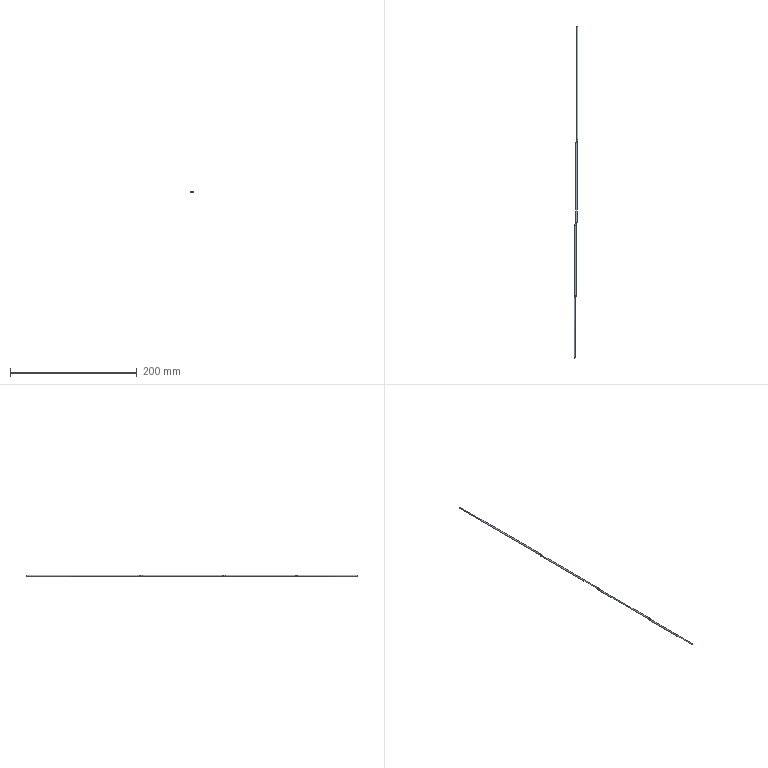Part | STEP file | 1-56.24 | 1 solid | 12 faces | box 5.973 x 524.553 x 2 mm | volume 1650 mm3 | torus 6 | cylinder 4 | plane 2 | commonest cylinder face diameters 2 x4
STEP:
#1=CARTESIAN_POINT('',(0.,0.,0.));
#2=DIRECTION('',(0.,0.,1.));
#3=DIRECTION('',(1.,0.,0.));
#4=AXIS2_PLACEMENT_3D('',#1,#2,#3);
#5=CARTESIAN_POINT('',(1.,0.,0.));
#6=VERTEX_POINT('',#5);
#7=CARTESIAN_POINT('',(0.,0.,0.));
#8=DIRECTION('',(0.,-1.,0.));
#9=DIRECTION('',(1.,0.,0.));
#10=AXIS2_PLACEMENT_3D('',#7,#8,#9);
#11=CIRCLE('',#10,1.);
#12=CARTESIAN_POINT('',(0.,0.,0.));
#13=DIRECTION('',(0.,-1.,0.));
#14=DIRECTION('',(0.,0.,-1.));
#15=AXIS2_PLACEMENT_3D('',#12,#13,#14);
#16=PLANE('',#15);
#17=CARTESIAN_POINT('',(0.,0.));
#18=DIRECTION('',(0.,1.));
#19=AXIS2_PLACEMENT_2D('',#17,#18);
#20=CIRCLE('',#19,1.);
#21=(GEOMETRIC_REPRESENTATION_CONTEXT(2)PARAMETRIC_REPRESENTATION_CONTEXT()REPRESENTATION_CONTEXT('',''));
#22=DEFINITIONAL_REPRESENTATION('',(#20),#21);
#23=PCURVE('',#16,#22);
#24=CARTESIAN_POINT('',(0.,0.,0.));
#25=DIRECTION('',(0.,1.,0.));
#26=DIRECTION('',(1.,0.,0.));
#27=AXIS2_PLACEMENT_3D('',#24,#25,#26);
#28=CYLINDRICAL_SURFACE('',#27,1.);
#29=CARTESIAN_POINT('',(6.283,0.));
#30=DIRECTION('',(-1.,0.));
#31=VECTOR('',#30,1.);
#32=LINE('',#29,#31);
#33=(GEOMETRIC_REPRESENTATION_CONTEXT(2)PARAMETRIC_REPRESENTATION_CONTEXT()REPRESENTATION_CONTEXT('',''));
#34=DEFINITIONAL_REPRESENTATION('',(#32),#33);
#35=PCURVE('',#28,#34);
#36=SURFACE_CURVE('',#11,(#23,#35),.PCURVE_S1.);
#37=EDGE_CURVE('',#6,#6,#36,.T.);
#38=ORIENTED_EDGE('',*,*,#37,.T.);
#39=EDGE_LOOP('',(#38));
#40=FACE_BOUND('',#39,.T.);
#41=ADVANCED_FACE('',(#40),#16,.T.);
#42=CARTESIAN_POINT('',(4.973,524.553,0.));
#43=VERTEX_POINT('',#42);
#44=CARTESIAN_POINT('',(3.973,524.553,0.));
#45=DIRECTION('',(0.,1.,0.));
#46=DIRECTION('',(1.,0.,0.));
#47=AXIS2_PLACEMENT_3D('',#44,#45,#46);
#48=CIRCLE('',#47,1.);
#49=CARTESIAN_POINT('',(3.973,524.553,0.));
#50=DIRECTION('',(0.,1.,0.));
#51=DIRECTION('',(1.,0.,0.));
#52=AXIS2_PLACEMENT_3D('',#49,#50,#51);
#53=PLANE('',#52);
#54=CARTESIAN_POINT('',(0.,0.));
#55=DIRECTION('',(1.,0.));
#56=AXIS2_PLACEMENT_2D('',#54,#55);
#57=CIRCLE('',#56,1.);
#58=(GEOMETRIC_REPRESENTATION_CONTEXT(2)PARAMETRIC_REPRESENTATION_CONTEXT()REPRESENTATION_CONTEXT('',''));
#59=DEFINITIONAL_REPRESENTATION('',(#57),#58);
#60=PCURVE('',#53,#59);
#61=CARTESIAN_POINT('',(3.973,344.553,0.));
#62=DIRECTION('',(0.,1.,0.));
#63=DIRECTION('',(1.,0.,0.));
#64=AXIS2_PLACEMENT_3D('',#61,#62,#63);
#65=CYLINDRICAL_SURFACE('',#64,1.);
#66=CARTESIAN_POINT('',(0.,180.));
#67=DIRECTION('',(1.,0.));
#68=VECTOR('',#67,1.);
#69=LINE('',#66,#68);
#70=(GEOMETRIC_REPRESENTATION_CONTEXT(2)PARAMETRIC_REPRESENTATION_CONTEXT()REPRESENTATION_CONTEXT('',''));
#71=DEFINITIONAL_REPRESENTATION('',(#69),#70);
#72=PCURVE('',#65,#71);
#73=SURFACE_CURVE('',#48,(#60,#72),.PCURVE_S1.);
#74=EDGE_CURVE('',#43,#43,#73,.T.);
#75=ORIENTED_EDGE('',*,*,#74,.T.);
#76=EDGE_LOOP('',(#75));
#77=FACE_BOUND('',#76,.T.);
#78=ADVANCED_FACE('',(#77),#53,.T.);
#79=ORIENTED_EDGE('',*,*,#37,.F.);
#80=CARTESIAN_POINT('',(1.,95.,0.));
#81=VERTEX_POINT('',#80);
#82=CARTESIAN_POINT('',(1.,0.,0.));
#83=DIRECTION('',(0.,1.,0.));
#84=VECTOR('',#83,1.);
#85=LINE('',#82,#84);
#86=CARTESIAN_POINT('',(6.283,0.));
#87=DIRECTION('',(0.,1.));
#88=VECTOR('',#87,1.);
#89=LINE('',#86,#88);
#90=(GEOMETRIC_REPRESENTATION_CONTEXT(2)PARAMETRIC_REPRESENTATION_CONTEXT()REPRESENTATION_CONTEXT('',''));
#91=DEFINITIONAL_REPRESENTATION('',(#89),#90);
#92=PCURVE('',#28,#91);
#93=CARTESIAN_POINT('',(0.,0.));
#94=DIRECTION('',(0.,1.));
#95=VECTOR('',#94,1.);
#96=LINE('',#93,#95);
#97=(GEOMETRIC_REPRESENTATION_CONTEXT(2)PARAMETRIC_REPRESENTATION_CONTEXT()REPRESENTATION_CONTEXT('',''));
#98=DEFINITIONAL_REPRESENTATION('',(#96),#97);
#99=PCURVE('',#28,#98);
#100=SEAM_CURVE('',#85,(#92,#99),.PCURVE_S1.);
#101=EDGE_CURVE('',#6,#81,#100,.T.);
#102=ORIENTED_EDGE('',*,*,#101,.T.);
#103=CARTESIAN_POINT('',(0.,95.,-1.));
#104=VERTEX_POINT('',#103);
#105=CARTESIAN_POINT('',(0.,95.,0.));
#106=DIRECTION('',(0.,1.,0.));
#107=DIRECTION('',(0.,0.,-1.));
#108=AXIS2_PLACEMENT_3D('',#105,#106,#107);
#109=CIRCLE('',#108,1.);
#110=CARTESIAN_POINT('',(1.571,95.));
#111=DIRECTION('',(1.,0.));
#112=VECTOR('',#111,1.);
#113=LINE('',#110,#112);
#114=(GEOMETRIC_REPRESENTATION_CONTEXT(2)PARAMETRIC_REPRESENTATION_CONTEXT()REPRESENTATION_CONTEXT('',''));
#115=DEFINITIONAL_REPRESENTATION('',(#113),#114);
#116=PCURVE('',#28,#115);
#117=CARTESIAN_POINT('',(2.72,95.,0.));
#118=DIRECTION('',(0.,0.,1.));
#119=DIRECTION('',(-1.,0.,0.));
#120=AXIS2_PLACEMENT_3D('',#117,#118,#119);
#121=TOROIDAL_SURFACE('',#120,2.72,1.);
#122=CARTESIAN_POINT('',(6.283,-1.571));
#123=DIRECTION('',(0.,1.));
#124=VECTOR('',#123,1.);
#125=LINE('',#122,#124);
#126=(GEOMETRIC_REPRESENTATION_CONTEXT(2)PARAMETRIC_REPRESENTATION_CONTEXT()REPRESENTATION_CONTEXT('',''));
#127=DEFINITIONAL_REPRESENTATION('',(#125),#126);
#128=PCURVE('',#121,#127);
#129=SURFACE_CURVE('',#109,(#116,#128),.PCURVE_S1.);
#130=EDGE_CURVE('',#104,#81,#129,.T.);
#131=ORIENTED_EDGE('',*,*,#130,.F.);
#132=CARTESIAN_POINT('',(0.,95.,0.));
#133=DIRECTION('',(0.,1.,0.));
#134=DIRECTION('',(1.,0.,0.));
#135=AXIS2_PLACEMENT_3D('',#132,#133,#134);
#136=CIRCLE('',#135,1.);
#137=CARTESIAN_POINT('',(0.,95.));
#138=DIRECTION('',(1.,0.));
#139=VECTOR('',#138,1.);
#140=LINE('',#137,#139);
#141=(GEOMETRIC_REPRESENTATION_CONTEXT(2)PARAMETRIC_REPRESENTATION_CONTEXT()REPRESENTATION_CONTEXT('',''));
#142=DEFINITIONAL_REPRESENTATION('',(#140),#141);
#143=PCURVE('',#28,#142);
#144=CARTESIAN_POINT('',(6.283,3.142));
#145=DIRECTION('',(0.,1.));
#146=VECTOR('',#145,1.);
#147=LINE('',#144,#146);
#148=(GEOMETRIC_REPRESENTATION_CONTEXT(2)PARAMETRIC_REPRESENTATION_CONTEXT()REPRESENTATION_CONTEXT('',''));
#149=DEFINITIONAL_REPRESENTATION('',(#147),#148);
#150=PCURVE('',#121,#149);
#151=SURFACE_CURVE('',#136,(#143,#150),.PCURVE_S1.);
#152=EDGE_CURVE('',#81,#104,#151,.T.);
#153=ORIENTED_EDGE('',*,*,#152,.F.);
#154=ORIENTED_EDGE('',*,*,#101,.F.);
#155=EDGE_LOOP('',(#79,#102,#131,#153,#154));
#156=FACE_BOUND('',#155,.T.);
#157=ADVANCED_FACE('',(#156),#28,.T.);
#158=ORIENTED_EDGE('',*,*,#130,.T.);
#159=ORIENTED_EDGE('',*,*,#152,.T.);
#160=CARTESIAN_POINT('',(0.6313,96.742,-1.));
#161=VERTEX_POINT('',#160);
#162=CARTESIAN_POINT('',(2.72,95.,-1.));
#163=DIRECTION('',(0.,0.,-1.));
#164=DIRECTION('',(-1.,0.,0.));
#165=AXIS2_PLACEMENT_3D('',#162,#163,#164);
#166=CIRCLE('',#165,2.72);
#167=CARTESIAN_POINT('',(6.283,4.712));
#168=DIRECTION('',(-1.,0.));
#169=VECTOR('',#168,1.);
#170=LINE('',#167,#169);
#171=(GEOMETRIC_REPRESENTATION_CONTEXT(2)PARAMETRIC_REPRESENTATION_CONTEXT()REPRESENTATION_CONTEXT('',''));
#172=DEFINITIONAL_REPRESENTATION('',(#170),#171);
#173=PCURVE('',#121,#172);
#174=CARTESIAN_POINT('',(6.283,-1.571));
#175=DIRECTION('',(-1.,0.));
#176=VECTOR('',#175,1.);
#177=LINE('',#174,#176);
#178=(GEOMETRIC_REPRESENTATION_CONTEXT(2)PARAMETRIC_REPRESENTATION_CONTEXT()REPRESENTATION_CONTEXT('',''));
#179=DEFINITIONAL_REPRESENTATION('',(#177),#178);
#180=PCURVE('',#121,#179);
#181=SEAM_CURVE('',#166,(#173,#180),.PCURVE_S1.);
#182=EDGE_CURVE('',#104,#161,#181,.T.);
#183=ORIENTED_EDGE('',*,*,#182,.T.);
#184=CARTESIAN_POINT('',(0.6313,96.742,0.));
#185=DIRECTION('',(-0.6406,-0.7679,0.));
#186=DIRECTION('',(0.,0.,-1.));
#187=AXIS2_PLACEMENT_3D('',#184,#185,#186);
#188=CIRCLE('',#187,1.);
#189=CARTESIAN_POINT('',(5.588,4.712));
#190=DIRECTION('',(0.,-1.));
#191=VECTOR('',#190,1.);
#192=LINE('',#189,#191);
#193=(GEOMETRIC_REPRESENTATION_CONTEXT(2)PARAMETRIC_REPRESENTATION_CONTEXT()REPRESENTATION_CONTEXT('',''));
#194=DEFINITIONAL_REPRESENTATION('',(#192),#193);
#195=PCURVE('',#121,#194);
#196=CARTESIAN_POINT('',(-1.301,98.354,0.));
#197=DIRECTION('',(0.,0.,-1.));
#198=DIRECTION('',(0.7679,-0.6406,0.));
#199=AXIS2_PLACEMENT_3D('',#196,#197,#198);
#200=TOROIDAL_SURFACE('',#199,2.516,1.);
#201=CARTESIAN_POINT('',(6.283,7.854));
#202=DIRECTION('',(0.,-1.));
#203=VECTOR('',#202,1.);
#204=LINE('',#201,#203);
#205=(GEOMETRIC_REPRESENTATION_CONTEXT(2)PARAMETRIC_REPRESENTATION_CONTEXT()REPRESENTATION_CONTEXT('',''));
#206=DEFINITIONAL_REPRESENTATION('',(#204),#205);
#207=PCURVE('',#200,#206);
#208=SURFACE_CURVE('',#188,(#195,#207),.PCURVE_S1.);
#209=EDGE_CURVE('',#161,#161,#208,.T.);
#210=ORIENTED_EDGE('',*,*,#209,.T.);
#211=ORIENTED_EDGE('',*,*,#182,.F.);
#212=EDGE_LOOP('',(#158,#159,#183,#210,#211));
#213=FACE_BOUND('',#212,.T.);
#214=ADVANCED_FACE('',(#213),#121,.T.);
#215=ORIENTED_EDGE('',*,*,#209,.F.);
#216=CARTESIAN_POINT('',(1.215,98.354,-1.));
#217=VERTEX_POINT('',#216);
#218=CARTESIAN_POINT('',(-1.301,98.354,-1.));
#219=DIRECTION('',(0.,0.,1.));
#220=DIRECTION('',(0.7679,-0.6406,0.));
#221=AXIS2_PLACEMENT_3D('',#218,#219,#220);
#222=CIRCLE('',#221,2.516);
#223=CARTESIAN_POINT('',(6.283,7.854));
#224=DIRECTION('',(-1.,0.));
#225=VECTOR('',#224,1.);
#226=LINE('',#223,#225);
#227=(GEOMETRIC_REPRESENTATION_CONTEXT(2)PARAMETRIC_REPRESENTATION_CONTEXT()REPRESENTATION_CONTEXT('',''));
#228=DEFINITIONAL_REPRESENTATION('',(#226),#227);
#229=PCURVE('',#200,#228);
#230=CARTESIAN_POINT('',(6.283,1.571));
#231=DIRECTION('',(-1.,0.));
#232=VECTOR('',#231,1.);
#233=LINE('',#230,#232);
#234=(GEOMETRIC_REPRESENTATION_CONTEXT(2)PARAMETRIC_REPRESENTATION_CONTEXT()REPRESENTATION_CONTEXT('',''));
#235=DEFINITIONAL_REPRESENTATION('',(#233),#234);
#236=PCURVE('',#200,#235);
#237=SEAM_CURVE('',#222,(#229,#236),.PCURVE_S1.);
#238=EDGE_CURVE('',#161,#217,#237,.T.);
#239=ORIENTED_EDGE('',*,*,#238,.T.);
#240=CARTESIAN_POINT('',(2.215,98.354,0.));
#241=VERTEX_POINT('',#240);
#242=CARTESIAN_POINT('',(1.215,98.354,0.));
#243=DIRECTION('',(0.,-1.,0.));
#244=DIRECTION('',(0.,0.,-1.));
#245=AXIS2_PLACEMENT_3D('',#242,#243,#244);
#246=CIRCLE('',#245,1.);
#247=CARTESIAN_POINT('',(5.588,7.854));
#248=DIRECTION('',(0.,-1.));
#249=VECTOR('',#248,1.);
#250=LINE('',#247,#249);
#251=(GEOMETRIC_REPRESENTATION_CONTEXT(2)PARAMETRIC_REPRESENTATION_CONTEXT()REPRESENTATION_CONTEXT('',''));
#252=DEFINITIONAL_REPRESENTATION('',(#250),#251);
#253=PCURVE('',#200,#252);
#254=CARTESIAN_POINT('',(1.215,98.354,0.));
#255=DIRECTION('',(0.,1.,0.));
#256=DIRECTION('',(1.,0.,0.));
#257=AXIS2_PLACEMENT_3D('',#254,#255,#256);
#258=CYLINDRICAL_SURFACE('',#257,1.);
#259=CARTESIAN_POINT('',(1.571,0.));
#260=DIRECTION('',(-1.,0.));
#261=VECTOR('',#260,1.);
#262=LINE('',#259,#261);
#263=(GEOMETRIC_REPRESENTATION_CONTEXT(2)PARAMETRIC_REPRESENTATION_CONTEXT()REPRESENTATION_CONTEXT('',''));
#264=DEFINITIONAL_REPRESENTATION('',(#262),#263);
#265=PCURVE('',#258,#264);
#266=SURFACE_CURVE('',#246,(#253,#265),.PCURVE_S1.);
#267=EDGE_CURVE('',#217,#241,#266,.T.);
#268=ORIENTED_EDGE('',*,*,#267,.T.);
#269=CARTESIAN_POINT('',(1.215,98.354,0.));
#270=DIRECTION('',(0.,-1.,0.));
#271=DIRECTION('',(1.,0.,0.));
#272=AXIS2_PLACEMENT_3D('',#269,#270,#271);
#273=CIRCLE('',#272,1.);
#274=CARTESIAN_POINT('',(5.588,6.283));
#275=DIRECTION('',(0.,-1.));
#276=VECTOR('',#275,1.);
#277=LINE('',#274,#276);
#278=(GEOMETRIC_REPRESENTATION_CONTEXT(2)PARAMETRIC_REPRESENTATION_CONTEXT()REPRESENTATION_CONTEXT('',''));
#279=DEFINITIONAL_REPRESENTATION('',(#277),#278);
#280=PCURVE('',#200,#279);
#281=CARTESIAN_POINT('',(6.283,0.));
#282=DIRECTION('',(-1.,0.));
#283=VECTOR('',#282,1.);
#284=LINE('',#281,#283);
#285=(GEOMETRIC_REPRESENTATION_CONTEXT(2)PARAMETRIC_REPRESENTATION_CONTEXT()REPRESENTATION_CONTEXT('',''));
#286=DEFINITIONAL_REPRESENTATION('',(#284),#285);
#287=PCURVE('',#258,#286);
#288=SURFACE_CURVE('',#273,(#280,#287),.PCURVE_S1.);
#289=EDGE_CURVE('',#241,#217,#288,.T.);
#290=ORIENTED_EDGE('',*,*,#289,.T.);
#291=ORIENTED_EDGE('',*,*,#238,.F.);
#292=EDGE_LOOP('',(#215,#239,#268,#290,#291));
#293=FACE_BOUND('',#292,.T.);
#294=ADVANCED_FACE('',(#293),#200,.T.);
#295=ORIENTED_EDGE('',*,*,#267,.F.);
#296=ORIENTED_EDGE('',*,*,#289,.F.);
#297=CARTESIAN_POINT('',(2.215,210.,0.));
#298=VERTEX_POINT('',#297);
#299=CARTESIAN_POINT('',(2.215,98.354,0.));
#300=DIRECTION('',(0.,1.,0.));
#301=VECTOR('',#300,1.);
#302=LINE('',#299,#301);
#303=CARTESIAN_POINT('',(6.283,0.));
#304=DIRECTION('',(0.,1.));
#305=VECTOR('',#304,1.);
#306=LINE('',#303,#305);
#307=(GEOMETRIC_REPRESENTATION_CONTEXT(2)PARAMETRIC_REPRESENTATION_CONTEXT()REPRESENTATION_CONTEXT('',''));
#308=DEFINITIONAL_REPRESENTATION('',(#306),#307);
#309=PCURVE('',#258,#308);
#310=CARTESIAN_POINT('',(0.,0.));
#311=DIRECTION('',(0.,1.));
#312=VECTOR('',#311,1.);
#313=LINE('',#310,#312);
#314=(GEOMETRIC_REPRESENTATION_CONTEXT(2)PARAMETRIC_REPRESENTATION_CONTEXT()REPRESENTATION_CONTEXT('',''));
#315=DEFINITIONAL_REPRESENTATION('',(#313),#314);
#316=PCURVE('',#258,#315);
#317=SEAM_CURVE('',#302,(#309,#316),.PCURVE_S1.);
#318=EDGE_CURVE('',#241,#298,#317,.T.);
#319=ORIENTED_EDGE('',*,*,#318,.T.);
#320=CARTESIAN_POINT('',(1.215,210.,-1.));
#321=VERTEX_POINT('',#320);
#322=CARTESIAN_POINT('',(1.215,210.,0.));
#323=DIRECTION('',(0.,1.,0.));
#324=DIRECTION('',(0.,0.,-1.));
#325=AXIS2_PLACEMENT_3D('',#322,#323,#324);
#326=CIRCLE('',#325,1.);
#327=CARTESIAN_POINT('',(1.571,111.646));
#328=DIRECTION('',(1.,0.));
#329=VECTOR('',#328,1.);
#330=LINE('',#327,#329);
#331=(GEOMETRIC_REPRESENTATION_CONTEXT(2)PARAMETRIC_REPRESENTATION_CONTEXT()REPRESENTATION_CONTEXT('',''));
#332=DEFINITIONAL_REPRESENTATION('',(#330),#331);
#333=PCURVE('',#258,#332);
#334=CARTESIAN_POINT('',(5.335,210.,0.));
#335=DIRECTION('',(0.,0.,1.));
#336=DIRECTION('',(-1.,0.,0.));
#337=AXIS2_PLACEMENT_3D('',#334,#335,#336);
#338=TOROIDAL_SURFACE('',#337,4.12,1.);
#339=CARTESIAN_POINT('',(6.283,-1.571));
#340=DIRECTION('',(0.,1.));
#341=VECTOR('',#340,1.);
#342=LINE('',#339,#341);
#343=(GEOMETRIC_REPRESENTATION_CONTEXT(2)PARAMETRIC_REPRESENTATION_CONTEXT()REPRESENTATION_CONTEXT('',''));
#344=DEFINITIONAL_REPRESENTATION('',(#342),#343);
#345=PCURVE('',#338,#344);
#346=SURFACE_CURVE('',#326,(#333,#345),.PCURVE_S1.);
#347=EDGE_CURVE('',#321,#298,#346,.T.);
#348=ORIENTED_EDGE('',*,*,#347,.F.);
#349=CARTESIAN_POINT('',(1.215,210.,0.));
#350=DIRECTION('',(0.,1.,0.));
#351=DIRECTION('',(1.,0.,0.));
#352=AXIS2_PLACEMENT_3D('',#349,#350,#351);
#353=CIRCLE('',#352,1.);
#354=CARTESIAN_POINT('',(0.,111.646));
#355=DIRECTION('',(1.,0.));
#356=VECTOR('',#355,1.);
#357=LINE('',#354,#356);
#358=(GEOMETRIC_REPRESENTATION_CONTEXT(2)PARAMETRIC_REPRESENTATION_CONTEXT()REPRESENTATION_CONTEXT('',''));
#359=DEFINITIONAL_REPRESENTATION('',(#357),#358);
#360=PCURVE('',#258,#359);
#361=CARTESIAN_POINT('',(6.283,3.142));
#362=DIRECTION('',(0.,1.));
#363=VECTOR('',#362,1.);
#364=LINE('',#361,#363);
#365=(GEOMETRIC_REPRESENTATION_CONTEXT(2)PARAMETRIC_REPRESENTATION_CONTEXT()REPRESENTATION_CONTEXT('',''));
#366=DEFINITIONAL_REPRESENTATION('',(#364),#365);
#367=PCURVE('',#338,#366);
#368=SURFACE_CURVE('',#353,(#360,#367),.PCURVE_S1.);
#369=EDGE_CURVE('',#298,#321,#368,.T.);
#370=ORIENTED_EDGE('',*,*,#369,.F.);
#371=ORIENTED_EDGE('',*,*,#318,.F.);
#372=EDGE_LOOP('',(#295,#296,#319,#348,#370,#371));
#373=FACE_BOUND('',#372,.T.);
#374=ADVANCED_FACE('',(#373),#258,.T.);
#375=ORIENTED_EDGE('',*,*,#347,.T.);
#376=ORIENTED_EDGE('',*,*,#369,.T.);
#377=CARTESIAN_POINT('',(1.87,212.228,-1.));
#378=VERTEX_POINT('',#377);
#379=CARTESIAN_POINT('',(5.335,210.,-1.));
#380=DIRECTION('',(0.,0.,-1.));
#381=DIRECTION('',(-1.,0.,0.));
#382=AXIS2_PLACEMENT_3D('',#379,#380,#381);
#383=CIRCLE('',#382,4.12);
#384=CARTESIAN_POINT('',(6.283,4.712));
#385=DIRECTION('',(-1.,0.));
#386=VECTOR('',#385,1.);
#387=LINE('',#384,#386);
#388=(GEOMETRIC_REPRESENTATION_CONTEXT(2)PARAMETRIC_REPRESENTATION_CONTEXT()REPRESENTATION_CONTEXT('',''));
#389=DEFINITIONAL_REPRESENTATION('',(#387),#388);
#390=PCURVE('',#338,#389);
#391=CARTESIAN_POINT('',(6.283,-1.571));
#392=DIRECTION('',(-1.,0.));
#393=VECTOR('',#392,1.);
#394=LINE('',#391,#393);
#395=(GEOMETRIC_REPRESENTATION_CONTEXT(2)PARAMETRIC_REPRESENTATION_CONTEXT()REPRESENTATION_CONTEXT('',''));
#396=DEFINITIONAL_REPRESENTATION('',(#394),#395);
#397=PCURVE('',#338,#396);
#398=SEAM_CURVE('',#383,(#390,#397),.PCURVE_S1.);
#399=EDGE_CURVE('',#321,#378,#398,.T.);
#400=ORIENTED_EDGE('',*,*,#399,.T.);
#401=CARTESIAN_POINT('',(1.87,212.228,0.));
#402=DIRECTION('',(-0.5407,-0.8412,0.));
#403=DIRECTION('',(0.,0.,-1.));
#404=AXIS2_PLACEMENT_3D('',#401,#402,#403);
#405=CIRCLE('',#404,1.);
#406=CARTESIAN_POINT('',(5.712,4.712));
#407=DIRECTION('',(0.,-1.));
#408=VECTOR('',#407,1.);
#409=LINE('',#406,#408);
#410=(GEOMETRIC_REPRESENTATION_CONTEXT(2)PARAMETRIC_REPRESENTATION_CONTEXT()REPRESENTATION_CONTEXT('',''));
#411=DEFINITIONAL_REPRESENTATION('',(#409),#410);
#412=PCURVE('',#338,#411);
#413=CARTESIAN_POINT('',(-2.211,214.851,0.));
#414=DIRECTION('',(0.,0.,-1.));
#415=DIRECTION('',(0.8412,-0.5407,0.));
#416=AXIS2_PLACEMENT_3D('',#413,#414,#415);
#417=TOROIDAL_SURFACE('',#416,4.851,1.);
#418=CARTESIAN_POINT('',(6.283,7.854));
#419=DIRECTION('',(0.,-1.));
#420=VECTOR('',#419,1.);
#421=LINE('',#418,#420);
#422=(GEOMETRIC_REPRESENTATION_CONTEXT(2)PARAMETRIC_REPRESENTATION_CONTEXT()REPRESENTATION_CONTEXT('',''));
#423=DEFINITIONAL_REPRESENTATION('',(#421),#422);
#424=PCURVE('',#417,#423);
#425=SURFACE_CURVE('',#405,(#412,#424),.PCURVE_S1.);
#426=EDGE_CURVE('',#378,#378,#425,.T.);
#427=ORIENTED_EDGE('',*,*,#426,.T.);
#428=ORIENTED_EDGE('',*,*,#399,.F.);
#429=EDGE_LOOP('',(#375,#376,#400,#427,#428));
#430=FACE_BOUND('',#429,.T.);
#431=ADVANCED_FACE('',(#430),#338,.T.);
#432=ORIENTED_EDGE('',*,*,#426,.F.);
#433=CARTESIAN_POINT('',(2.64,214.851,-1.));
#434=VERTEX_POINT('',#433);
#435=CARTESIAN_POINT('',(-2.211,214.851,-1.));
#436=DIRECTION('',(0.,0.,1.));
#437=DIRECTION('',(0.8412,-0.5407,0.));
#438=AXIS2_PLACEMENT_3D('',#435,#436,#437);
#439=CIRCLE('',#438,4.851);
#440=CARTESIAN_POINT('',(6.283,7.854));
#441=DIRECTION('',(-1.,0.));
#442=VECTOR('',#441,1.);
#443=LINE('',#440,#442);
#444=(GEOMETRIC_REPRESENTATION_CONTEXT(2)PARAMETRIC_REPRESENTATION_CONTEXT()REPRESENTATION_CONTEXT('',''));
#445=DEFINITIONAL_REPRESENTATION('',(#443),#444);
#446=PCURVE('',#417,#445);
#447=CARTESIAN_POINT('',(6.283,1.571));
#448=DIRECTION('',(-1.,0.));
#449=VECTOR('',#448,1.);
#450=LINE('',#447,#449);
#451=(GEOMETRIC_REPRESENTATION_CONTEXT(2)PARAMETRIC_REPRESENTATION_CONTEXT()REPRESENTATION_CONTEXT('',''));
#452=DEFINITIONAL_REPRESENTATION('',(#450),#451);
#453=PCURVE('',#417,#452);
#454=SEAM_CURVE('',#439,(#446,#453),.PCURVE_S1.);
#455=EDGE_CURVE('',#378,#434,#454,.T.);
#456=ORIENTED_EDGE('',*,*,#455,.T.);
#457=CARTESIAN_POINT('',(3.64,214.851,0.));
#458=VERTEX_POINT('',#457);
#459=CARTESIAN_POINT('',(2.64,214.851,0.));
#460=DIRECTION('',(0.,-1.,0.));
#461=DIRECTION('',(0.,0.,-1.));
#462=AXIS2_PLACEMENT_3D('',#459,#460,#461);
#463=CIRCLE('',#462,1.);
#464=CARTESIAN_POINT('',(5.712,7.854));
#465=DIRECTION('',(0.,-1.));
#466=VECTOR('',#465,1.);
#467=LINE('',#464,#466);
#468=(GEOMETRIC_REPRESENTATION_CONTEXT(2)PARAMETRIC_REPRESENTATION_CONTEXT()REPRESENTATION_CONTEXT('',''));
#469=DEFINITIONAL_REPRESENTATION('',(#467),#468);
#470=PCURVE('',#417,#469);
#471=CARTESIAN_POINT('',(2.64,214.851,0.));
#472=DIRECTION('',(0.,1.,0.));
#473=DIRECTION('',(1.,0.,0.));
#474=AXIS2_PLACEMENT_3D('',#471,#472,#473);
#475=CYLINDRICAL_SURFACE('',#474,1.);
#476=CARTESIAN_POINT('',(1.571,0.));
#477=DIRECTION('',(-1.,0.));
#478=VECTOR('',#477,1.);
#479=LINE('',#476,#478);
#480=(GEOMETRIC_REPRESENTATION_CONTEXT(2)PARAMETRIC_REPRESENTATION_CONTEXT()REPRESENTATION_CONTEXT('',''));
#481=DEFINITIONAL_REPRESENTATION('',(#479),#480);
#482=PCURVE('',#475,#481);
#483=SURFACE_CURVE('',#463,(#470,#482),.PCURVE_S1.);
#484=EDGE_CURVE('',#434,#458,#483,.T.);
#485=ORIENTED_EDGE('',*,*,#484,.T.);
#486=CARTESIAN_POINT('',(2.64,214.851,0.));
#487=DIRECTION('',(0.,-1.,0.));
#488=DIRECTION('',(1.,0.,0.));
#489=AXIS2_PLACEMENT_3D('',#486,#487,#488);
#490=CIRCLE('',#489,1.);
#491=CARTESIAN_POINT('',(5.712,6.283));
#492=DIRECTION('',(0.,-1.));
#493=VECTOR('',#492,1.);
#494=LINE('',#491,#493);
#495=(GEOMETRIC_REPRESENTATION_CONTEXT(2)PARAMETRIC_REPRESENTATION_CONTEXT()REPRESENTATION_CONTEXT('',''));
#496=DEFINITIONAL_REPRESENTATION('',(#494),#495);
#497=PCURVE('',#417,#496);
#498=CARTESIAN_POINT('',(6.283,0.));
#499=DIRECTION('',(-1.,0.));
#500=VECTOR('',#499,1.);
#501=LINE('',#498,#500);
#502=(GEOMETRIC_REPRESENTATION_CONTEXT(2)PARAMETRIC_REPRESENTATION_CONTEXT()REPRESENTATION_CONTEXT('',''));
#503=DEFINITIONAL_REPRESENTATION('',(#501),#502);
#504=PCURVE('',#475,#503);
#505=SURFACE_CURVE('',#490,(#497,#504),.PCURVE_S1.);
#506=EDGE_CURVE('',#458,#434,#505,.T.);
#507=ORIENTED_EDGE('',*,*,#506,.T.);
#508=ORIENTED_EDGE('',*,*,#455,.F.);
#509=EDGE_LOOP('',(#432,#456,#485,#507,#508));
#510=FACE_BOUND('',#509,.T.);
#511=ADVANCED_FACE('',(#510),#417,.T.);
#512=ORIENTED_EDGE('',*,*,#484,.F.);
#513=ORIENTED_EDGE('',*,*,#506,.F.);
#514=CARTESIAN_POINT('',(3.64,339.851,0.));
#515=VERTEX_POINT('',#514);
#516=CARTESIAN_POINT('',(3.64,214.851,0.));
#517=DIRECTION('',(0.,1.,0.));
#518=VECTOR('',#517,1.);
#519=LINE('',#516,#518);
#520=CARTESIAN_POINT('',(6.283,0.));
#521=DIRECTION('',(0.,1.));
#522=VECTOR('',#521,1.);
#523=LINE('',#520,#522);
#524=(GEOMETRIC_REPRESENTATION_CONTEXT(2)PARAMETRIC_REPRESENTATION_CONTEXT()REPRESENTATION_CONTEXT('',''));
#525=DEFINITIONAL_REPRESENTATION('',(#523),#524);
#526=PCURVE('',#475,#525);
#527=CARTESIAN_POINT('',(0.,0.));
#528=DIRECTION('',(0.,1.));
#529=VECTOR('',#528,1.);
#530=LINE('',#527,#529);
#531=(GEOMETRIC_REPRESENTATION_CONTEXT(2)PARAMETRIC_REPRESENTATION_CONTEXT()REPRESENTATION_CONTEXT('',''));
#532=DEFINITIONAL_REPRESENTATION('',(#530),#531);
#533=PCURVE('',#475,#532);
#534=SEAM_CURVE('',#519,(#526,#533),.PCURVE_S1.);
#535=EDGE_CURVE('',#458,#515,#534,.T.);
#536=ORIENTED_EDGE('',*,*,#535,.T.);
#537=CARTESIAN_POINT('',(2.64,339.851,-1.));
#538=VERTEX_POINT('',#537);
#539=CARTESIAN_POINT('',(2.64,339.851,0.));
#540=DIRECTION('',(0.,1.,0.));
#541=DIRECTION('',(0.,0.,-1.));
#542=AXIS2_PLACEMENT_3D('',#539,#540,#541);
#543=CIRCLE('',#542,1.);
#544=CARTESIAN_POINT('',(1.571,125.));
#545=DIRECTION('',(1.,0.));
#546=VECTOR('',#545,1.);
#547=LINE('',#544,#546);
#548=(GEOMETRIC_REPRESENTATION_CONTEXT(2)PARAMETRIC_REPRESENTATION_CONTEXT()REPRESENTATION_CONTEXT('',''));
#549=DEFINITIONAL_REPRESENTATION('',(#547),#548);
#550=PCURVE('',#475,#549);
#551=CARTESIAN_POINT('',(7.673,339.851,0.));
#552=DIRECTION('',(0.,0.,1.));
#553=DIRECTION('',(-1.,0.,0.));
#554=AXIS2_PLACEMENT_3D('',#551,#552,#553);
#555=TOROIDAL_SURFACE('',#554,5.033,1.);
#556=CARTESIAN_POINT('',(6.283,-1.571));
#557=DIRECTION('',(0.,1.));
#558=VECTOR('',#557,1.);
#559=LINE('',#556,#558);
#560=(GEOMETRIC_REPRESENTATION_CONTEXT(2)PARAMETRIC_REPRESENTATION_CONTEXT()REPRESENTATION_CONTEXT('',''));
#561=DEFINITIONAL_REPRESENTATION('',(#559),#560);
#562=PCURVE('',#555,#561);
#563=SURFACE_CURVE('',#543,(#550,#562),.PCURVE_S1.);
#564=EDGE_CURVE('',#538,#515,#563,.T.);
#565=ORIENTED_EDGE('',*,*,#564,.F.);
#566=CARTESIAN_POINT('',(2.64,339.851,0.));
#567=DIRECTION('',(0.,1.,0.));
#568=DIRECTION('',(1.,0.,0.));
#569=AXIS2_PLACEMENT_3D('',#566,#567,#568);
#570=CIRCLE('',#569,1.);
#571=CARTESIAN_POINT('',(0.,125.));
#572=DIRECTION('',(1.,0.));
#573=VECTOR('',#572,1.);
#574=LINE('',#571,#573);
#575=(GEOMETRIC_REPRESENTATION_CONTEXT(2)PARAMETRIC_REPRESENTATION_CONTEXT()REPRESENTATION_CONTEXT('',''));
#576=DEFINITIONAL_REPRESENTATION('',(#574),#575);
#577=PCURVE('',#475,#576);
#578=CARTESIAN_POINT('',(6.283,3.142));
#579=DIRECTION('',(0.,1.));
#580=VECTOR('',#579,1.);
#581=LINE('',#578,#580);
#582=(GEOMETRIC_REPRESENTATION_CONTEXT(2)PARAMETRIC_REPRESENTATION_CONTEXT()REPRESENTATION_CONTEXT('',''));
#583=DEFINITIONAL_REPRESENTATION('',(#581),#582);
#584=PCURVE('',#555,#583);
#585=SURFACE_CURVE('',#570,(#577,#584),.PCURVE_S1.);
#586=EDGE_CURVE('',#515,#538,#585,.T.);
#587=ORIENTED_EDGE('',*,*,#586,.F.);
#588=ORIENTED_EDGE('',*,*,#535,.F.);
#589=EDGE_LOOP('',(#512,#513,#536,#565,#587,#588));
#590=FACE_BOUND('',#589,.T.);
#591=ADVANCED_FACE('',(#590),#475,.T.);
#592=ORIENTED_EDGE('',*,*,#564,.T.);
#593=ORIENTED_EDGE('',*,*,#586,.T.);
#594=CARTESIAN_POINT('',(3.389,342.492,-1.));
#595=VERTEX_POINT('',#594);
#596=CARTESIAN_POINT('',(7.673,339.851,-1.));
#597=DIRECTION('',(0.,0.,-1.));
#598=DIRECTION('',(-1.,0.,0.));
#599=AXIS2_PLACEMENT_3D('',#596,#597,#598);
#600=CIRCLE('',#599,5.033);
#601=CARTESIAN_POINT('',(6.283,4.712));
#602=DIRECTION('',(-1.,0.));
#603=VECTOR('',#602,1.);
#604=LINE('',#601,#603);
#605=(GEOMETRIC_REPRESENTATION_CONTEXT(2)PARAMETRIC_REPRESENTATION_CONTEXT()REPRESENTATION_CONTEXT('',''));
#606=DEFINITIONAL_REPRESENTATION('',(#604),#605);
#607=PCURVE('',#555,#606);
#608=CARTESIAN_POINT('',(6.283,-1.571));
#609=DIRECTION('',(-1.,0.));
#610=VECTOR('',#609,1.);
#611=LINE('',#608,#610);
#612=(GEOMETRIC_REPRESENTATION_CONTEXT(2)PARAMETRIC_REPRESENTATION_CONTEXT()REPRESENTATION_CONTEXT('',''));
#613=DEFINITIONAL_REPRESENTATION('',(#611),#612);
#614=PCURVE('',#555,#613);
#615=SEAM_CURVE('',#600,(#607,#614),.PCURVE_S1.);
#616=EDGE_CURVE('',#538,#595,#615,.T.);
#617=ORIENTED_EDGE('',*,*,#616,.T.);
#618=CARTESIAN_POINT('',(3.389,342.492,0.));
#619=DIRECTION('',(-0.5247,-0.8513,0.));
#620=DIRECTION('',(0.,0.,-1.));
#621=AXIS2_PLACEMENT_3D('',#618,#619,#620);
#622=CIRCLE('',#621,1.);
#623=CARTESIAN_POINT('',(5.731,4.712));
#624=DIRECTION('',(0.,-1.));
#625=VECTOR('',#624,1.);
#626=LINE('',#623,#625);
#627=(GEOMETRIC_REPRESENTATION_CONTEXT(2)PARAMETRIC_REPRESENTATION_CONTEXT()REPRESENTATION_CONTEXT('',''));
#628=DEFINITIONAL_REPRESENTATION('',(#626),#627);
#629=PCURVE('',#555,#628);
#630=CARTESIAN_POINT('',(0.04353,344.553,0.));
#631=DIRECTION('',(0.,0.,-1.));
#632=DIRECTION('',(0.8513,-0.5247,0.));
#633=AXIS2_PLACEMENT_3D('',#630,#631,#632);
#634=TOROIDAL_SURFACE('',#633,3.929,1.);
#635=CARTESIAN_POINT('',(6.283,7.854));
#636=DIRECTION('',(0.,-1.));
#637=VECTOR('',#636,1.);
#638=LINE('',#635,#637);
#639=(GEOMETRIC_REPRESENTATION_CONTEXT(2)PARAMETRIC_REPRESENTATION_CONTEXT()REPRESENTATION_CONTEXT('',''));
#640=DEFINITIONAL_REPRESENTATION('',(#638),#639);
#641=PCURVE('',#634,#640);
#642=SURFACE_CURVE('',#622,(#629,#641),.PCURVE_S1.);
#643=EDGE_CURVE('',#595,#595,#642,.T.);
#644=ORIENTED_EDGE('',*,*,#643,.T.);
#645=ORIENTED_EDGE('',*,*,#616,.F.);
#646=EDGE_LOOP('',(#592,#593,#617,#644,#645));
#647=FACE_BOUND('',#646,.T.);
#648=ADVANCED_FACE('',(#647),#555,.T.);
#649=ORIENTED_EDGE('',*,*,#643,.F.);
#650=CARTESIAN_POINT('',(3.973,344.553,-1.));
#651=VERTEX_POINT('',#650);
#652=CARTESIAN_POINT('',(0.04353,344.553,-1.));
#653=DIRECTION('',(0.,0.,1.));
#654=DIRECTION('',(0.8513,-0.5247,0.));
#655=AXIS2_PLACEMENT_3D('',#652,#653,#654);
#656=CIRCLE('',#655,3.929);
#657=CARTESIAN_POINT('',(6.283,7.854));
#658=DIRECTION('',(-1.,0.));
#659=VECTOR('',#658,1.);
#660=LINE('',#657,#659);
#661=(GEOMETRIC_REPRESENTATION_CONTEXT(2)PARAMETRIC_REPRESENTATION_CONTEXT()REPRESENTATION_CONTEXT('',''));
#662=DEFINITIONAL_REPRESENTATION('',(#660),#661);
#663=PCURVE('',#634,#662);
#664=CARTESIAN_POINT('',(6.283,1.571));
#665=DIRECTION('',(-1.,0.));
#666=VECTOR('',#665,1.);
#667=LINE('',#664,#666);
#668=(GEOMETRIC_REPRESENTATION_CONTEXT(2)PARAMETRIC_REPRESENTATION_CONTEXT()REPRESENTATION_CONTEXT('',''));
#669=DEFINITIONAL_REPRESENTATION('',(#667),#668);
#670=PCURVE('',#634,#669);
#671=SEAM_CURVE('',#656,(#663,#670),.PCURVE_S1.);
#672=EDGE_CURVE('',#595,#651,#671,.T.);
#673=ORIENTED_EDGE('',*,*,#672,.T.);
#674=CARTESIAN_POINT('',(4.973,344.553,0.));
#675=VERTEX_POINT('',#674);
#676=CARTESIAN_POINT('',(3.973,344.553,0.));
#677=DIRECTION('',(0.,-1.,0.));
#678=DIRECTION('',(0.,0.,-1.));
#679=AXIS2_PLACEMENT_3D('',#676,#677,#678);
#680=CIRCLE('',#679,1.);
#681=CARTESIAN_POINT('',(5.731,7.854));
#682=DIRECTION('',(0.,-1.));
#683=VECTOR('',#682,1.);
#684=LINE('',#681,#683);
#685=(GEOMETRIC_REPRESENTATION_CONTEXT(2)PARAMETRIC_REPRESENTATION_CONTEXT()REPRESENTATION_CONTEXT('',''));
#686=DEFINITIONAL_REPRESENTATION('',(#684),#685);
#687=PCURVE('',#634,#686);
#688=CARTESIAN_POINT('',(1.571,0.));
#689=DIRECTION('',(-1.,0.));
#690=VECTOR('',#689,1.);
#691=LINE('',#688,#690);
#692=(GEOMETRIC_REPRESENTATION_CONTEXT(2)PARAMETRIC_REPRESENTATION_CONTEXT()REPRESENTATION_CONTEXT('',''));
#693=DEFINITIONAL_REPRESENTATION('',(#691),#692);
#694=PCURVE('',#65,#693);
#695=SURFACE_CURVE('',#680,(#687,#694),.PCURVE_S1.);
#696=EDGE_CURVE('',#651,#675,#695,.T.);
#697=ORIENTED_EDGE('',*,*,#696,.T.);
#698=CARTESIAN_POINT('',(3.973,344.553,0.));
#699=DIRECTION('',(0.,-1.,0.));
#700=DIRECTION('',(1.,0.,0.));
#701=AXIS2_PLACEMENT_3D('',#698,#699,#700);
#702=CIRCLE('',#701,1.);
#703=CARTESIAN_POINT('',(5.731,6.283));
#704=DIRECTION('',(0.,-1.));
#705=VECTOR('',#704,1.);
#706=LINE('',#703,#705);
#707=(GEOMETRIC_REPRESENTATION_CONTEXT(2)PARAMETRIC_REPRESENTATION_CONTEXT()REPRESENTATION_CONTEXT('',''));
#708=DEFINITIONAL_REPRESENTATION('',(#706),#707);
#709=PCURVE('',#634,#708);
#710=CARTESIAN_POINT('',(6.283,0.));
#711=DIRECTION('',(-1.,0.));
#712=VECTOR('',#711,1.);
#713=LINE('',#710,#712);
#714=(GEOMETRIC_REPRESENTATION_CONTEXT(2)PARAMETRIC_REPRESENTATION_CONTEXT()REPRESENTATION_CONTEXT('',''));
#715=DEFINITIONAL_REPRESENTATION('',(#713),#714);
#716=PCURVE('',#65,#715);
#717=SURFACE_CURVE('',#702,(#709,#716),.PCURVE_S1.);
#718=EDGE_CURVE('',#675,#651,#717,.T.);
#719=ORIENTED_EDGE('',*,*,#718,.T.);
#720=ORIENTED_EDGE('',*,*,#672,.F.);
#721=EDGE_LOOP('',(#649,#673,#697,#719,#720));
#722=FACE_BOUND('',#721,.T.);
#723=ADVANCED_FACE('',(#722),#634,.T.);
#724=ORIENTED_EDGE('',*,*,#696,.F.);
#725=ORIENTED_EDGE('',*,*,#718,.F.);
#726=CARTESIAN_POINT('',(4.973,344.553,0.));
#727=DIRECTION('',(0.,1.,0.));
#728=VECTOR('',#727,1.);
#729=LINE('',#726,#728);
#730=CARTESIAN_POINT('',(6.283,0.));
#731=DIRECTION('',(0.,1.));
#732=VECTOR('',#731,1.);
#733=LINE('',#730,#732);
#734=(GEOMETRIC_REPRESENTATION_CONTEXT(2)PARAMETRIC_REPRESENTATION_CONTEXT()REPRESENTATION_CONTEXT('',''));
#735=DEFINITIONAL_REPRESENTATION('',(#733),#734);
#736=PCURVE('',#65,#735);
#737=CARTESIAN_POINT('',(0.,0.));
#738=DIRECTION('',(0.,1.));
#739=VECTOR('',#738,1.);
#740=LINE('',#737,#739);
#741=(GEOMETRIC_REPRESENTATION_CONTEXT(2)PARAMETRIC_REPRESENTATION_CONTEXT()REPRESENTATION_CONTEXT('',''));
#742=DEFINITIONAL_REPRESENTATION('',(#740),#741);
#743=PCURVE('',#65,#742);
#744=SEAM_CURVE('',#729,(#736,#743),.PCURVE_S1.);
#745=EDGE_CURVE('',#675,#43,#744,.T.);
#746=ORIENTED_EDGE('',*,*,#745,.T.);
#747=ORIENTED_EDGE('',*,*,#74,.F.);
#748=ORIENTED_EDGE('',*,*,#745,.F.);
#749=EDGE_LOOP('',(#724,#725,#746,#747,#748));
#750=FACE_BOUND('',#749,.T.);
#751=ADVANCED_FACE('',(#750),#65,.T.);
#752=CLOSED_SHELL('',(#41,#78,#157,#214,#294,#374,#431,#511,#591,#648,#723,#751));
#753=MANIFOLD_SOLID_BREP('',#752);
#754=(LENGTH_UNIT()NAMED_UNIT(*)SI_UNIT(.MILLI.,.METRE.));
#755=UNCERTAINTY_MEASURE_WITH_UNIT(LENGTH_MEASURE(0.0000001),#754,'','');
#756=(NAMED_UNIT(*)PLANE_ANGLE_UNIT()SI_UNIT($,.RADIAN.));
#757=(NAMED_UNIT(*)SI_UNIT($,.STERADIAN.)SOLID_ANGLE_UNIT());
#758=(GEOMETRIC_REPRESENTATION_CONTEXT(3)GLOBAL_UNCERTAINTY_ASSIGNED_CONTEXT((#755))GLOBAL_UNIT_ASSIGNED_CONTEXT((#754,#756,#757))REPRESENTATION_CONTEXT('',''));
#759=ADVANCED_BREP_SHAPE_REPRESENTATION('',(#4,#753),#758);